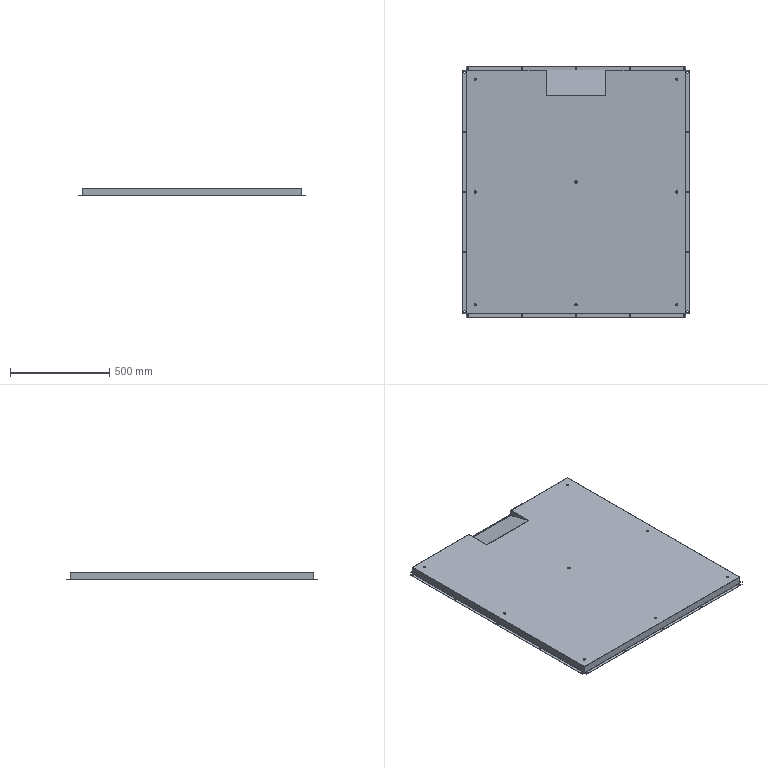Part | SolidWorks | 2 solids | 206 faces | box 1139 x 1259 x 40 mm | volume 1605167 mm3 | plane 106 | cylinder 88 | spline 12 | commonest cylinder face diameters 7 x50 11 x16 0.4 x11 2.4 x11